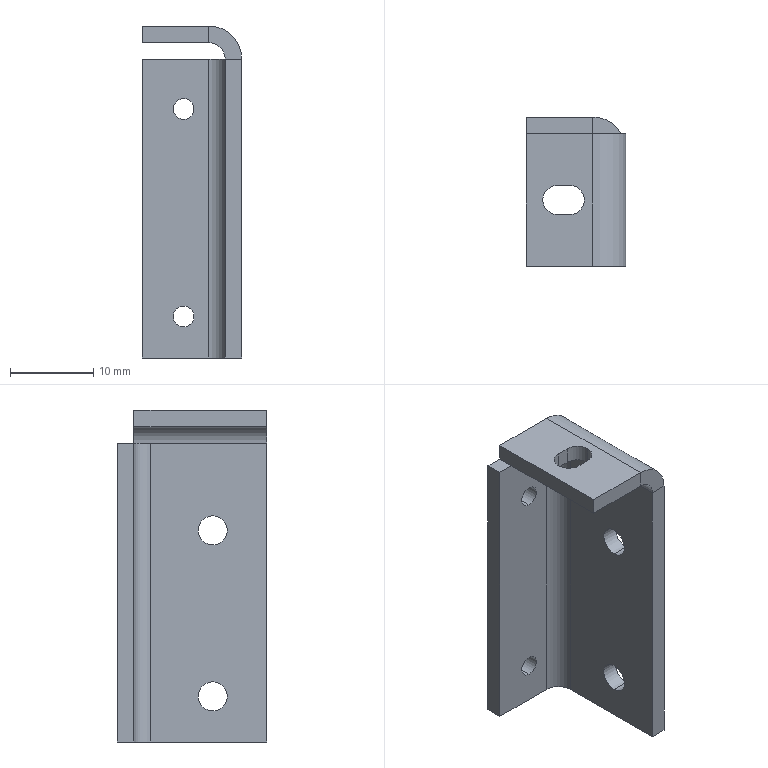Part | STEP file | MGN9 guide rail mounting angle 1001 | 1 solid | 36 faces | box 12 x 18 x 40 mm | volume 2242 mm3 | plane 21 | cylinder 15 | commonest cylinder face diameters 3.5 x7 2.5 x4 4 x2 8 x2